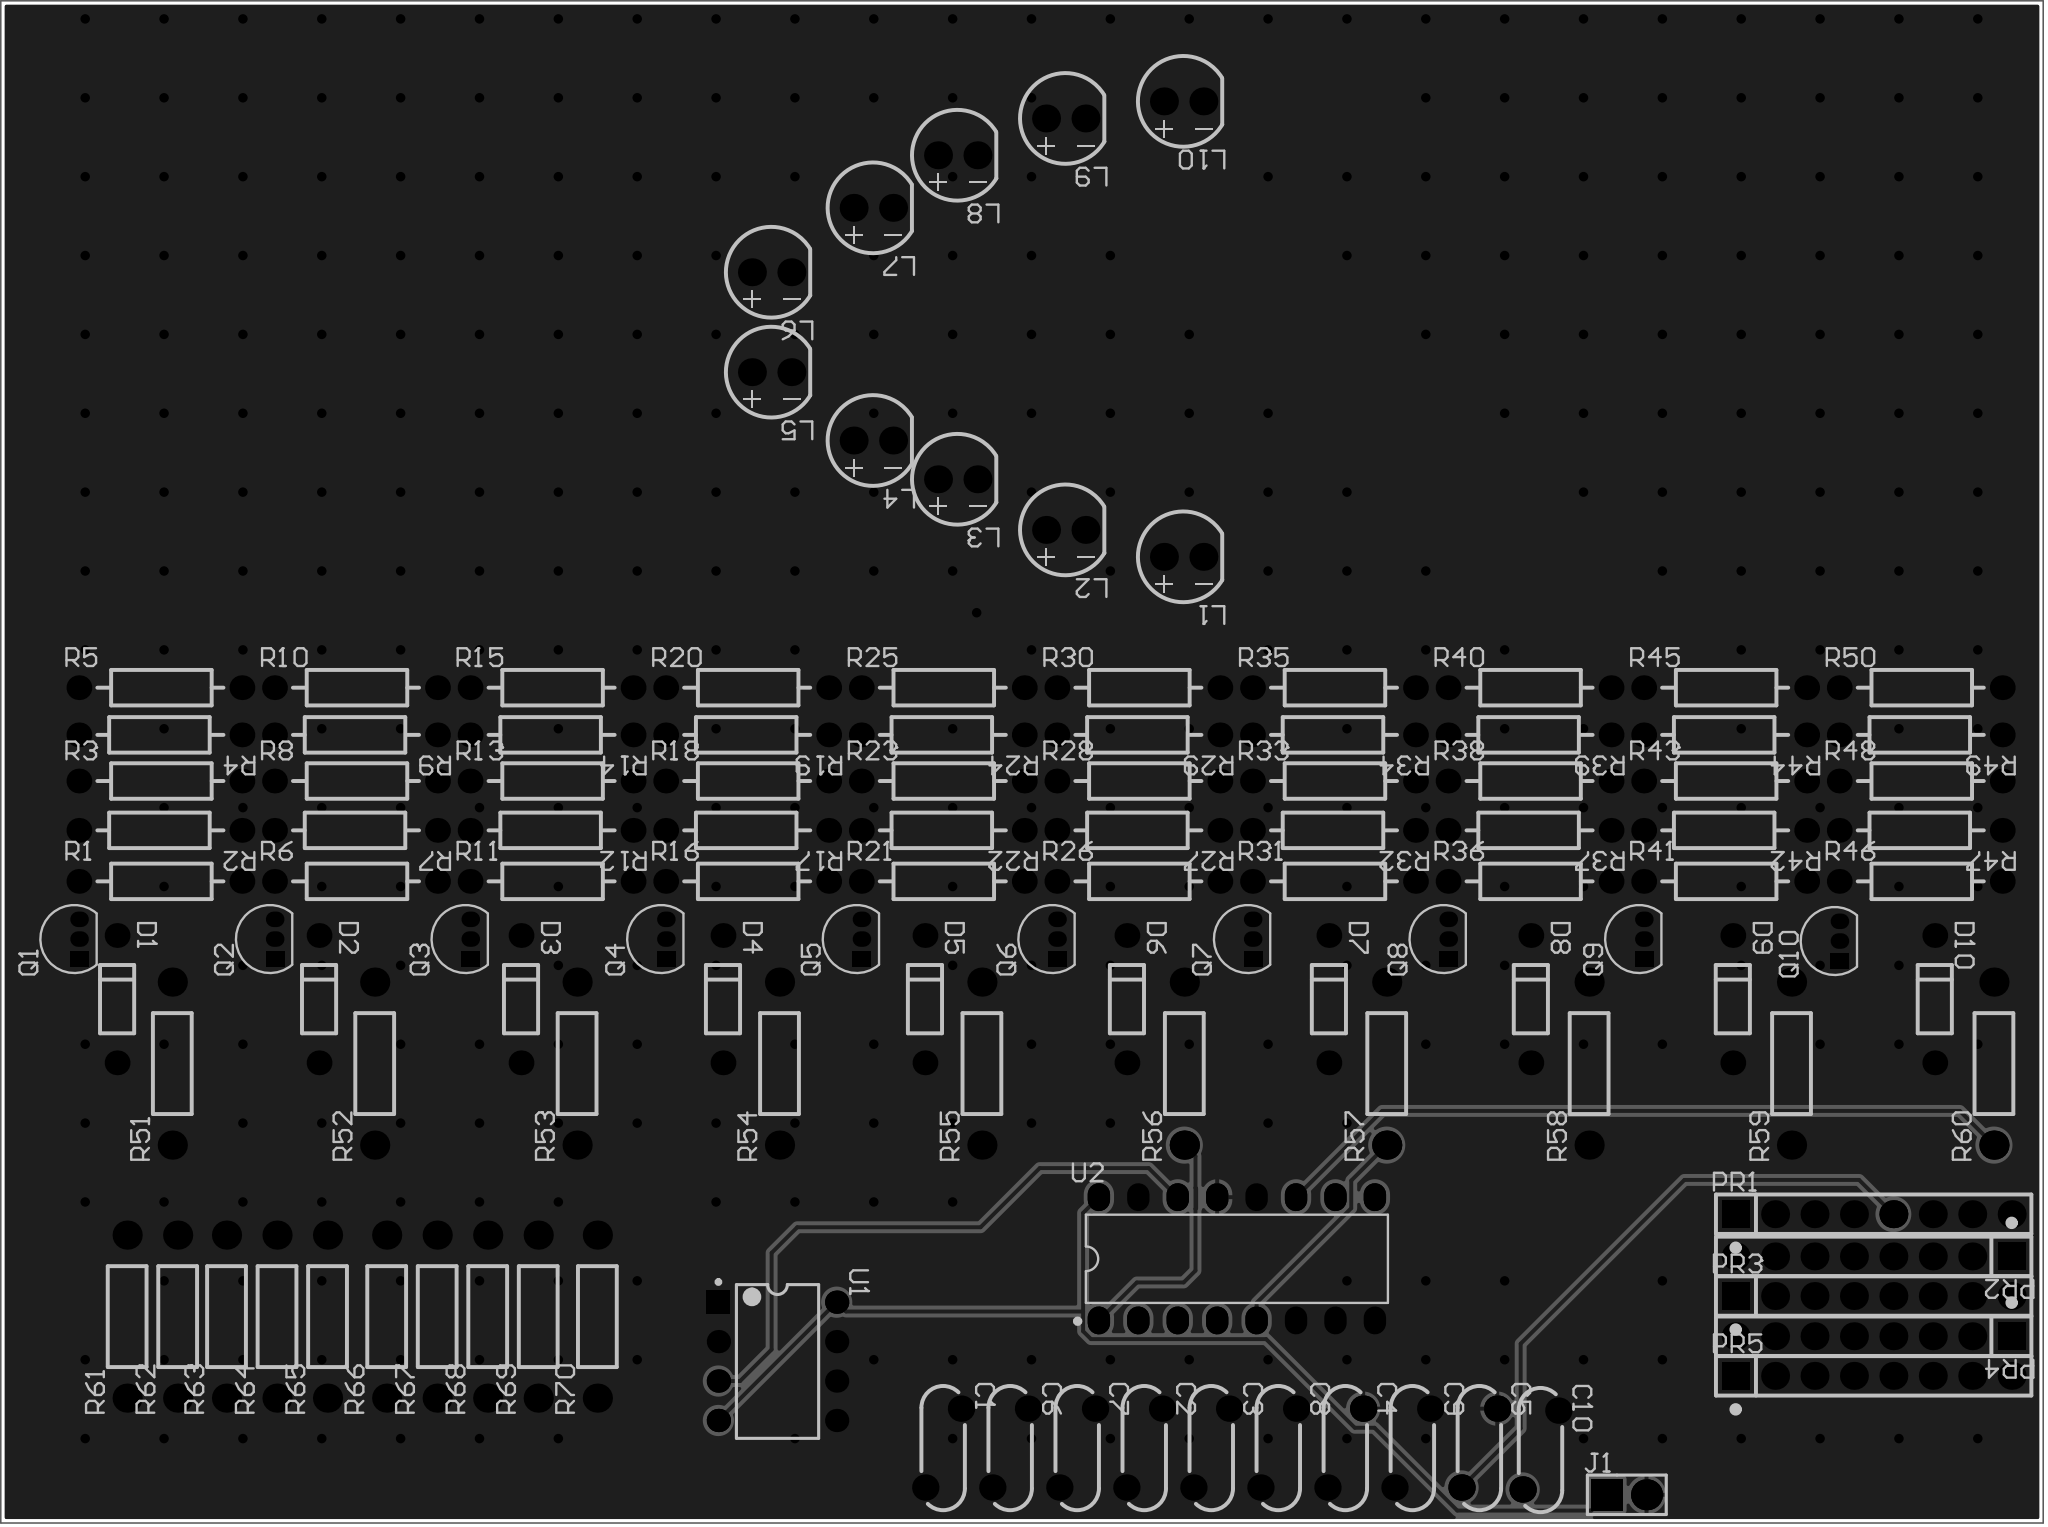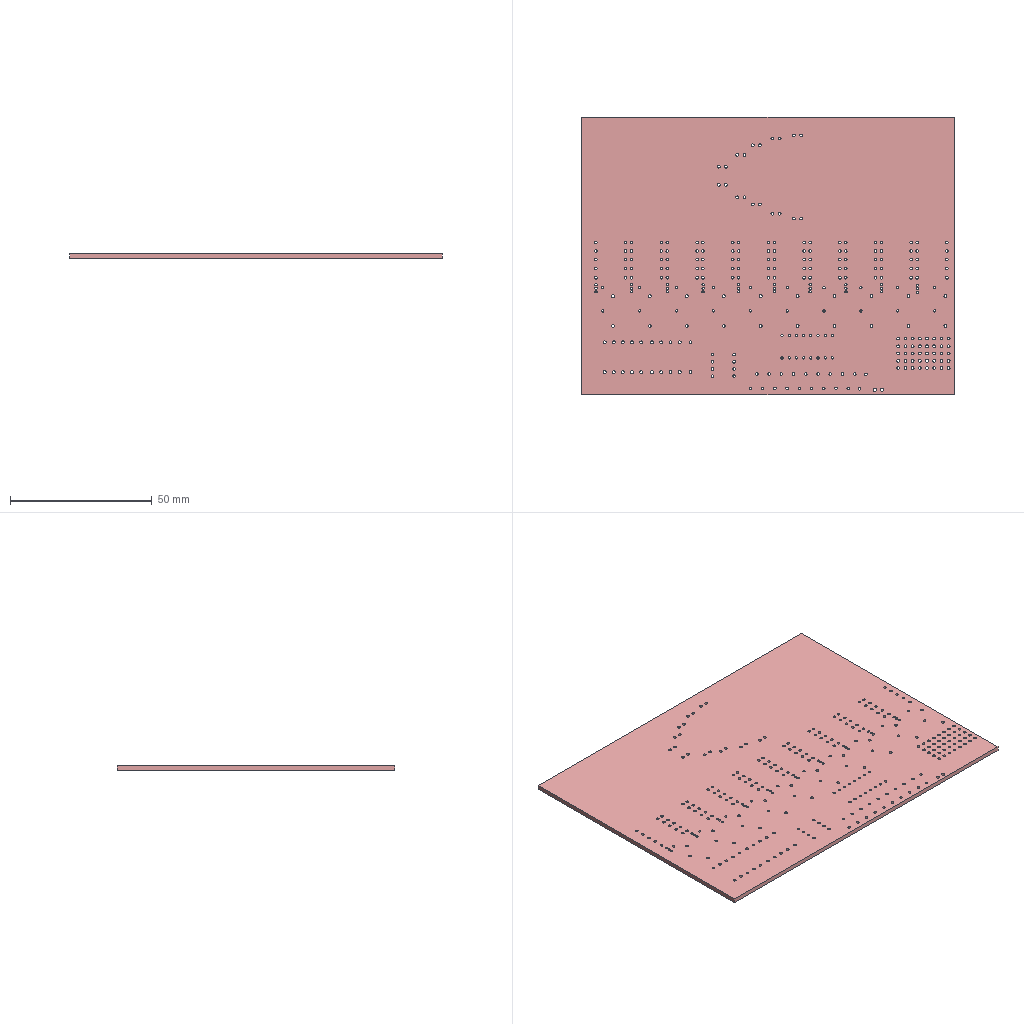Circuit board layout | Altium Designer | box 131.6 x 98 x 1.6 mm
Layer stack:
# Altium Designer layer stack of  (unit mm; dielectric type: 0 none, 1 core, 2 prepreg, 3 surface material)
index,name,kind,layer,copper_thickness_mm,dielectric_type,dielectric_thickness_mm,dielectric_material,dielectric_constant
0,Top Paste Mask Layer,other,,,,,,
1,Top Silkscreen Layer,other,,,,,,
2,Top Solder Mask Layer,dielectric,,,3,0.01,,3.3
3,Top Layer,copper,Top Layer,0.035,,,,
4,Dielectric1,dielectric,,,3,1.51,FR4,4.5
5,Bottom Layer,copper,Bottom Layer,0.035,,,,
6,Bottom Solder Mask Layer,dielectric,,,3,0.01,,3.3
7,Bottom Silkscreen Layer,other,,,,,,
8,Bottom Paste Mask Layer,other,,,,,,
# drill layer pairs: low layer,high layer
drill_pair,Top Layer,Bottom Layer
Part placement:
Designator,Comment,Layer,Footprint,Center-X(mm),Center-Y(mm),Rotation
C1,10nF,TopLayer,CAP-TH_L8.0-W2.8-P5.08-D0.6,143.51,88.9,270
C2,10nF,TopLayer,CAP-TH_L8.0-W2.8-P5.08-D0.6,156.464,88.9,270
C3,10nF,TopLayer,CAP-TH_L8.0-W2.8-P5.08-D0.6,160.782,88.9,270
C4,10nF,TopLayer,CAP-TH_L8.0-W2.8-P5.08-D0.6,169.418,88.9,270
C5,10nF,TopLayer,CAP-TH_L8.0-W2.8-P5.08-D0.6,178.054,88.9,270
C6,10nF,TopLayer,CAP-TH_L8.0-W2.8-P5.08-D0.6,147.828,88.9,270
C7,10nF,TopLayer,CAP-TH_L8.0-W2.8-P5.08-D0.6,152.146,88.9,270
C8,10nF,TopLayer,CAP-TH_L8.0-W2.8-P5.08-D0.6,165.1,88.9,270
C9,10nF,TopLayer,CAP-TH_L8.0-W2.8-P5.08-D0.6,173.736,88.9,270
C10,10nF,TopLayer,CAP-TH_L8.0-W2.8-P5.08-D0.6,181.991,88.773,270
D1,1N4148TR,TopLayer,DO-35_BD2.0-L4.2-P8.20-D0.5-RD,90.297,117.815,270
D2,1N4148TR,TopLayer,DO-35_BD2.0-L4.2-P8.20-D0.5-RD,103.307,117.815,270
D3,1N4148TR,TopLayer,DO-35_BD2.0-L4.2-P8.20-D0.5-RD,116.318,117.815,270
D4,1N4148TR,TopLayer,DO-35_BD2.0-L4.2-P8.20-D0.5-RD,129.328,117.815,270
D5,1N4148TR,TopLayer,DO-35_BD2.0-L4.2-P8.20-D0.5-RD,142.339,117.815,270
D6,1N4148TR,TopLayer,DO-35_BD2.0-L4.2-P8.20-D0.5-RD,155.349,117.815,270
D7,1N4148TR,TopLayer,DO-35_BD2.0-L4.2-P8.20-D0.5-RD,168.36,117.815,270
D8,1N4148TR,TopLayer,DO-35_BD2.0-L4.2-P8.20-D0.5-RD,181.37,117.815,270
D9,1N4148TR,TopLayer,DO-35_BD2.0-L4.2-P8.20-D0.5-RD,194.381,117.815,270
D10,1N4148TR,TopLayer,DO-35_BD2.0-L4.2-P8.20-D0.5-RD,207.391,117.815,270
J1,PZ254V-11-02P,TopLayer,HDR-TH_2P-P2.54-V-M,187.552,85.892,0
L1,XL-502SURD,TopLayer,LED-TH_BD5.9-P2.54-RD_RED,159.004,146.304,180
L2,XL-502SURD,TopLayer,LED-TH_BD5.9-P2.54-RD_RED,151.41,148.04,180
L3,XL-502SURD,TopLayer,LED-TH_BD5.9-P2.54-RD_RED,144.45,151.299,180
L4,XL-502SURD,TopLayer,LED-TH_BD5.9-P2.54-RD_RED,139.015,153.797,180
L5,XL-502SURD,TopLayer,LED-TH_BD5.9-P2.54-RD_RED,132.462,158.2,180
L6,XL-502SURD,TopLayer,LED-TH_BD5.9-P2.54-RD_RED,132.462,164.634,180
L7,XL-502SURD,TopLayer,LED-TH_BD5.9-P2.54-RD_RED,139.015,168.783,180
L8,XL-502SURD,TopLayer,LED-TH_BD5.9-P2.54-RD_RED,144.45,172.17,180
L9,XL-502SURD,TopLayer,LED-TH_BD5.9-P2.54-RD_RED,151.41,174.54,180
L10,XL-502SURD,TopLayer,LED-TH_BD5.9-P2.54-RD_RED,159.004,175.641,180
PR1,10kΩ,TopLayer,RES-ARRAY-TH_8P-L20.3-W2.5-P2.54,203.454,103.964,0
PR2,10kΩ,TopLayer,RES-ARRAY-TH_8P-L20.3-W2.5-P2.54,203.454,101.247,180
PR3,10kΩ,TopLayer,RES-ARRAY-TH_8P-L20.3-W2.5-P2.54,203.454,98.695,0
PR4,10kΩ,TopLayer,RES-ARRAY-TH_8P-L20.3-W2.5-P2.54,203.454,96.105,180
PR5,10kΩ,TopLayer,RES-ARRAY-TH_8P-L20.3-W2.5-P2.54,203.454,93.552,0
Q1,S8050,TopLayer,TO-92-3_L4.5-W3.5-P1.27-L,87.88,121.686,90
Q2,S8050,TopLayer,TO-92-3_L4.5-W3.5-P1.27-L,100.48,121.686,90
Q3,S8050,TopLayer,TO-92-3_L4.5-W3.5-P1.27-L,113.08,121.686,90
Q4,S8050,TopLayer,TO-92-3_L4.5-W3.5-P1.27-L,125.68,121.686,90
Q5,S8050,TopLayer,TO-92-3_L4.5-W3.5-P1.27-L,138.28,121.686,90
Q6,S8050,TopLayer,TO-92-3_L4.5-W3.5-P1.27-L,150.881,121.686,90
Q7,S8050,TopLayer,TO-92-3_L4.5-W3.5-P1.27-L,163.481,121.686,90
Q8,S8050,TopLayer,TO-92-3_L4.5-W3.5-P1.27-L,176.081,121.686,90
Q9,S8050,TopLayer,TO-92-3_L4.5-W3.5-P1.27-L,188.681,121.686,90
Q10,S8050,TopLayer,TO-92-3_L4.5-W3.5-P1.27-L,201.281,121.559,90
R1,100Ω,TopLayer,RES-TH_BD2.2-L6.5-P10.50-D0.6,93.087,125.402,0
R2,100Ω,TopLayer,RES-TH_BD2.2-L6.5-P10.50-D0.6,93.087,128.687,180
R3,100Ω,TopLayer,RES-TH_BD2.2-L6.5-P10.50-D0.6,93.087,131.865,0
R4,100Ω,TopLayer,RES-TH_BD2.2-L6.5-P10.50-D0.6,93.087,134.837,180
R5,100Ω,TopLayer,RES-TH_BD2.2-L6.5-P10.50-D0.6,93.087,137.877,0
R6,100Ω,TopLayer,RES-TH_BD2.2-L6.5-P10.50-D0.6,105.687,125.402,0
R7,100Ω,TopLayer,RES-TH_BD2.2-L6.5-P10.50-D0.6,105.687,128.687,180
R8,100Ω,TopLayer,RES-TH_BD2.2-L6.5-P10.50-D0.6,105.687,131.865,0
R9,100Ω,TopLayer,RES-TH_BD2.2-L6.5-P10.50-D0.6,105.687,134.837,180
R10,100Ω,TopLayer,RES-TH_BD2.2-L6.5-P10.50-D0.6,105.687,137.877,0
R11,100Ω,TopLayer,RES-TH_BD2.2-L6.5-P10.50-D0.6,118.287,125.402,0
R12,100Ω,TopLayer,RES-TH_BD2.2-L6.5-P10.50-D0.6,118.287,128.687,180
R13,100Ω,TopLayer,RES-TH_BD2.2-L6.5-P10.50-D0.6,118.287,131.865,0
R14,100Ω,TopLayer,RES-TH_BD2.2-L6.5-P10.50-D0.6,118.287,134.837,180
R15,100Ω,TopLayer,RES-TH_BD2.2-L6.5-P10.50-D0.6,118.287,137.877,0
R16,100Ω,TopLayer,RES-TH_BD2.2-L6.5-P10.50-D0.6,130.887,125.402,0
R17,100Ω,TopLayer,RES-TH_BD2.2-L6.5-P10.50-D0.6,130.887,128.687,180
R18,100Ω,TopLayer,RES-TH_BD2.2-L6.5-P10.50-D0.6,130.887,131.865,0
R19,100Ω,TopLayer,RES-TH_BD2.2-L6.5-P10.50-D0.6,130.887,134.837,180
R20,100Ω,TopLayer,RES-TH_BD2.2-L6.5-P10.50-D0.6,130.887,137.877,0
R21,100Ω,TopLayer,RES-TH_BD2.2-L6.5-P10.50-D0.6,143.487,125.402,0
R22,100Ω,TopLayer,RES-TH_BD2.2-L6.5-P10.50-D0.6,143.488,128.687,180
R23,100Ω,TopLayer,RES-TH_BD2.2-L6.5-P10.50-D0.6,143.487,131.865,0
R24,100Ω,TopLayer,RES-TH_BD2.2-L6.5-P10.50-D0.6,143.488,134.837,180
R25,100Ω,TopLayer,RES-TH_BD2.2-L6.5-P10.50-D0.6,143.487,137.877,0
R26,100Ω,TopLayer,RES-TH_BD2.2-L6.5-P10.50-D0.6,156.088,125.402,0
R27,100Ω,TopLayer,RES-TH_BD2.2-L6.5-P10.50-D0.6,156.088,128.687,180
R28,100Ω,TopLayer,RES-TH_BD2.2-L6.5-P10.50-D0.6,156.088,131.865,0
R29,100Ω,TopLayer,RES-TH_BD2.2-L6.5-P10.50-D0.6,156.088,134.837,180
R30,100Ω,TopLayer,RES-TH_BD2.2-L6.5-P10.50-D0.6,156.088,137.877,0
R31,100Ω,TopLayer,RES-TH_BD2.2-L6.5-P10.50-D0.6,168.688,125.402,0
R32,100Ω,TopLayer,RES-TH_BD2.2-L6.5-P10.50-D0.6,168.688,128.687,180
R33,100Ω,TopLayer,RES-TH_BD2.2-L6.5-P10.50-D0.6,168.688,131.865,0
R34,100Ω,TopLayer,RES-TH_BD2.2-L6.5-P10.50-D0.6,168.688,134.837,180
R35,100Ω,TopLayer,RES-TH_BD2.2-L6.5-P10.50-D0.6,168.688,137.877,0
R36,100Ω,TopLayer,RES-TH_BD2.2-L6.5-P10.50-D0.6,181.288,125.402,0
R37,100Ω,TopLayer,RES-TH_BD2.2-L6.5-P10.50-D0.6,181.288,128.687,180
R38,100Ω,TopLayer,RES-TH_BD2.2-L6.5-P10.50-D0.6,181.288,131.865,0
R39,100Ω,TopLayer,RES-TH_BD2.2-L6.5-P10.50-D0.6,181.288,134.837,180
R40,100Ω,TopLayer,RES-TH_BD2.2-L6.5-P10.50-D0.6,181.288,137.877,0
R41,100Ω,TopLayer,RES-TH_BD2.2-L6.5-P10.50-D0.6,193.888,125.402,0
R42,100Ω,TopLayer,RES-TH_BD2.2-L6.5-P10.50-D0.6,193.888,128.687,180
R43,100Ω,TopLayer,RES-TH_BD2.2-L6.5-P10.50-D0.6,193.888,131.865,0
R44,100Ω,TopLayer,RES-TH_BD2.2-L6.5-P10.50-D0.6,193.888,134.837,180
R45,100Ω,TopLayer,RES-TH_BD2.2-L6.5-P10.50-D0.6,193.888,137.877,0
R46,100Ω,TopLayer,RES-TH_BD2.2-L6.5-P10.50-D0.6,206.488,125.402,0
R47,100Ω,TopLayer,RES-TH_BD2.2-L6.5-P10.50-D0.6,206.488,128.687,180
R48,100Ω,TopLayer,RES-TH_BD2.2-L6.5-P10.50-D0.6,206.488,131.865,0
R49,100Ω,TopLayer,RES-TH_BD2.2-L6.5-P10.50-D0.6,206.488,134.837,180
R50,100Ω,TopLayer,RES-TH_BD2.2-L6.5-P10.50-D0.6,206.488,137.877,0
R51,1kΩ,TopLayer,RES-TH_BD2.5-L6.5-P10.50-D0.6,93.853,113.665,90
R52,1kΩ,TopLayer,RES-TH_BD2.5-L6.5-P10.50-D0.6,106.892,113.665,90
R53,1kΩ,TopLayer,RES-TH_BD2.5-L6.5-P10.50-D0.6,119.93,113.665,90
R54,1kΩ,TopLayer,RES-TH_BD2.5-L6.5-P10.50-D0.6,132.969,113.665,90
R55,1kΩ,TopLayer,RES-TH_BD2.5-L6.5-P10.50-D0.6,146.008,113.665,90
R56,1kΩ,TopLayer,RES-TH_BD2.5-L6.5-P10.50-D0.6,159.046,113.665,90
R57,1kΩ,TopLayer,RES-TH_BD2.5-L6.5-P10.50-D0.6,172.085,113.665,90
R58,1kΩ,TopLayer,RES-TH_BD2.5-L6.5-P10.50-D0.6,185.124,113.665,90
R59,1kΩ,TopLayer,RES-TH_BD2.5-L6.5-P10.50-D0.6,198.162,113.665,90
R60,1kΩ,TopLayer,RES-TH_BD2.5-L6.5-P10.50-D0.6,211.201,113.665,90
R61,1kΩ,TopLayer,RES-TH_BD2.5-L6.5-P10.50-D0.6,90.944,97.368,90
R62,1kΩ,TopLayer,RES-TH_BD2.5-L6.5-P10.50-D0.6,94.198,97.368,90
R63,1kΩ,TopLayer,RES-TH_BD2.5-L6.5-P10.50-D0.6,97.346,97.368,90
R64,1kΩ,TopLayer,RES-TH_BD2.5-L6.5-P10.50-D0.6,100.6,97.368,90
R65,1kΩ,TopLayer,RES-TH_BD2.5-L6.5-P10.50-D0.6,103.853,97.368,90
R66,1kΩ,TopLayer,RES-TH_BD2.5-L6.5-P10.50-D0.6,107.663,97.368,90
R67,1kΩ,TopLayer,RES-TH_BD2.5-L6.5-P10.50-D0.6,110.918,97.368,90
R68,1kΩ,TopLayer,RES-TH_BD2.5-L6.5-P10.50-D0.6,114.172,97.368,90
R69,1kΩ,TopLayer,RES-TH_BD2.5-L6.5-P10.50-D0.6,117.426,97.368,90
R70,1kΩ,TopLayer,RES-TH_BD2.5-L6.5-P10.50-D0.6,121.236,97.368,90
U1,NE555P,TopLayer,DIP-8_L9.8-W6.6-P2.54-LS7.6-BL,132.842,94.488,270
U2,CD4017CN,TopLayer,PDIP-16_L19.3-W6.4-P2.54-LS7.94-BL,162.433,101.092,0
Pad and via stacks:
# Altium Designer via and pad stacks of  (unit mm). Each distinct definition once, with the count of objects using it.
# via: kind,start_layer,end_layer,hole_mm,diameter_mm,mode(0 simple;1 top-mid-bottom;2 full stack),diameter_per_layer,count,example_net
# pad: kind,layer,hole_mm,hole_type(0 round;1 square;2 slot),plating,top_size,top_shape(1 round;2 rect;3 octagon;9 rounded rect),mid_size,bottom_size,mode,footprint,size_per_layer,count,example
pad,Multi-Layer,0.9,0,plated,1.7x1.7,1,1.7x1.7,1.7x1.7,0,CAP-TH_L8.0-W2.8-P5.08-D0.6,,20,C1.1
pad,Multi-Layer,0.8,0,plated,1.6x1.6,1,1.6x1.6,1.6x1.6,0,DO-35_BD2.0-L4.2-P8.20-D0.5-RD,,20,D1.2
pad,Multi-Layer,1.2,0,plated,2x2,2,2x2,2x2,0,HDR-TH_2P-P2.54-V-M,,1,J1.1
pad,Multi-Layer,1.2,0,plated,2x2,1,2x2,2x2,0,HDR-TH_2P-P2.54-V-M,,1,J1.2
pad,Multi-Layer,1,0,plated,1.8x1.8,1,1.8x1.8,1.8x1.8,0,LED-TH_BD5.9-P2.54-RD_RED,,20,L1.2
pad,Multi-Layer,1,0,plated,1.8x1.8,2,1.8x1.8,1.8x1.8,0,RES-ARRAY-TH_8P-L20.3-W2.5-P2.54,,5,PR1.1
pad,Multi-Layer,1,0,plated,1.8x1.8,1,1.8x1.8,1.8x1.8,0,RES-ARRAY-TH_8P-L20.3-W2.5-P2.54,,35,PR1.2
pad,Multi-Layer,0.7,2,plated,1x1.2,2,1x1.2,1x1.2,0,TO-92-3_L4.5-W3.5-P1.27-L,,10,Q1.1
pad,Multi-Layer,0.7,2,plated,1x1.2,1,1x1.2,1x1.2,0,TO-92-3_L4.5-W3.5-P1.27-L,,20,Q1.2
pad,Multi-Layer,0.9144,0,plated,1.6x1.6,1,1.6x1.6,1.6x1.6,0,RES-TH_BD2.2-L6.5-P10.50-D0.6,,100,R1.1
pad,Multi-Layer,1,0,plated,1.88x1.88,1,1.88x1.88,1.88x1.88,0,RES-TH_BD2.5-L6.5-P10.50-D0.6,,40,R51.1
pad,Multi-Layer,0.9,0,plated,1.5x1.5,2,1.5x1.5,1.5x1.5,0,DIP-8_L9.8-W6.6-P2.54-LS7.6-BL,,1,U1.1
pad,Multi-Layer,0.9,0,plated,1.5x1.5,1,1.5x1.5,1.5x1.5,0,DIP-8_L9.8-W6.6-P2.54-LS7.6-BL,,7,U1.2
pad,Multi-Layer,0.8,0,plated,1.44x1.8,1,1.44x1.8,1.44x1.8,0,PDIP-16_L19.3-W6.4-P2.54-LS7.94-BL,,16,U2.1
via,Top Layer,Bottom Layer,0.3048,0.61,0,,364,$1N7351
Copper pours:
name,layer,net,type(0 solid;1 hatched;2 none)
Bottom Layer-GND,Bottom Layer,GND,0
Top Layer-GND,Top Layer,GND,0